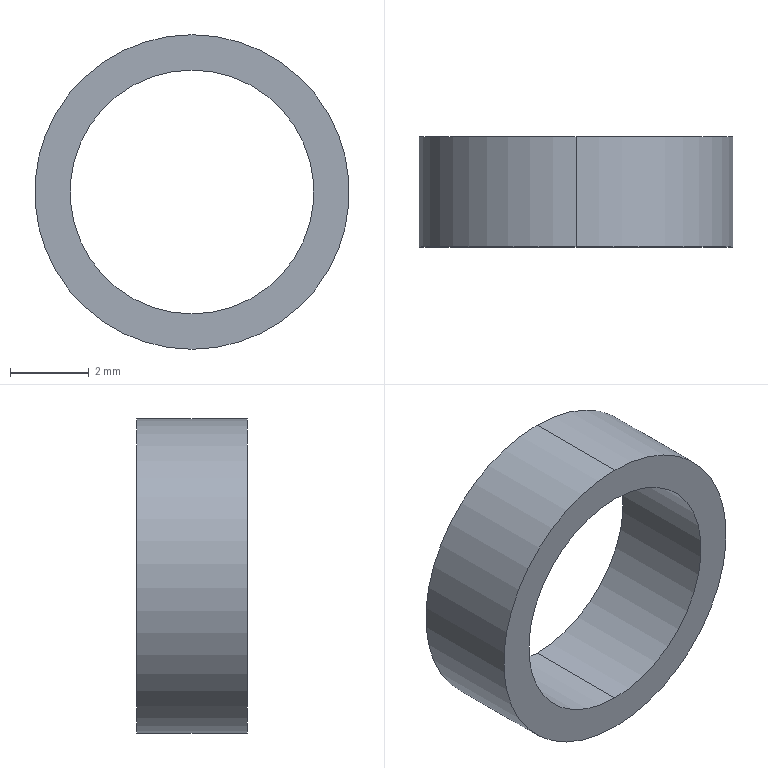Part | SolidWorks | features Extrusion 1 | 1 solid | 6 faces | box 8 x 2.8 x 8 mm | volume 56.209 mm3 | cylinder 4 | plane 2 | commonest cylinder face diameters 6.2 x2 8 x2
STEP:
#1=CARTESIAN_POINT('',(0.,2.8,-3.1));
#2=VERTEX_POINT('',#1);
#3=CARTESIAN_POINT('',(0.,2.8,3.1));
#4=VERTEX_POINT('',#3);
#5=CARTESIAN_POINT('',(0.,2.8,0.));
#6=DIRECTION('',(0.,1.,0.));
#7=DIRECTION('',(0.,0.,1.));
#8=AXIS2_PLACEMENT_3D('',#5,#6,#7);
#9=CIRCLE('',#8,3.1);
#10=EDGE_CURVE('',#2,#4,#9,.T.);
#11=ORIENTED_EDGE('',*,*,#10,.T.);
#12=CARTESIAN_POINT('',(0.,0.,3.1));
#13=VERTEX_POINT('',#12);
#14=CARTESIAN_POINT('',(0.,2.8,3.1));
#15=DIRECTION('',(0.,-1.,0.));
#16=VECTOR('',#15,1000.);
#17=LINE('',#14,#16);
#18=EDGE_CURVE('',#4,#13,#17,.T.);
#19=ORIENTED_EDGE('',*,*,#18,.T.);
#20=CARTESIAN_POINT('',(0.,0.,-3.1));
#21=VERTEX_POINT('',#20);
#22=CARTESIAN_POINT('',(0.,0.,0.));
#23=DIRECTION('',(0.,1.,0.));
#24=DIRECTION('',(0.,0.,1.));
#25=AXIS2_PLACEMENT_3D('',#22,#23,#24);
#26=CIRCLE('',#25,3.1);
#27=EDGE_CURVE('',#21,#13,#26,.T.);
#28=ORIENTED_EDGE('',*,*,#27,.F.);
#29=CARTESIAN_POINT('',(0.,2.8,-3.1));
#30=DIRECTION('',(0.,-1.,0.));
#31=VECTOR('',#30,1000.);
#32=LINE('',#29,#31);
#33=EDGE_CURVE('',#2,#21,#32,.T.);
#34=ORIENTED_EDGE('',*,*,#33,.F.);
#35=EDGE_LOOP('',(#11,#19,#28,#34));
#36=FACE_OUTER_BOUND('',#35,.T.);
#37=CARTESIAN_POINT('',(0.,2.8,0.));
#38=DIRECTION('',(0.,-1.,0.));
#39=DIRECTION('',(0.,0.,-1.));
#40=AXIS2_PLACEMENT_3D('',#37,#38,#39);
#41=CYLINDRICAL_SURFACE('',#40,3.1);
#42=ADVANCED_FACE('',(#36),#41,.F.);
#43=CARTESIAN_POINT('',(0.,2.8,4.));
#44=VERTEX_POINT('',#43);
#45=CARTESIAN_POINT('',(0.,2.8,-4.));
#46=VERTEX_POINT('',#45);
#47=CARTESIAN_POINT('',(0.,2.8,0.));
#48=DIRECTION('',(0.,1.,0.));
#49=DIRECTION('',(0.,0.,1.));
#50=AXIS2_PLACEMENT_3D('',#47,#48,#49);
#51=CIRCLE('',#50,4.);
#52=EDGE_CURVE('',#44,#46,#51,.T.);
#53=ORIENTED_EDGE('',*,*,#52,.F.);
#54=CARTESIAN_POINT('',(0.,0.,4.));
#55=VERTEX_POINT('',#54);
#56=CARTESIAN_POINT('',(0.,2.8,4.));
#57=DIRECTION('',(0.,-1.,0.));
#58=VECTOR('',#57,1000.);
#59=LINE('',#56,#58);
#60=EDGE_CURVE('',#44,#55,#59,.T.);
#61=ORIENTED_EDGE('',*,*,#60,.T.);
#62=CARTESIAN_POINT('',(0.,0.,-4.));
#63=VERTEX_POINT('',#62);
#64=CARTESIAN_POINT('',(0.,0.,0.));
#65=DIRECTION('',(0.,1.,0.));
#66=DIRECTION('',(0.,0.,1.));
#67=AXIS2_PLACEMENT_3D('',#64,#65,#66);
#68=CIRCLE('',#67,4.);
#69=EDGE_CURVE('',#55,#63,#68,.T.);
#70=ORIENTED_EDGE('',*,*,#69,.T.);
#71=CARTESIAN_POINT('',(0.,2.8,-4.));
#72=DIRECTION('',(0.,-1.,0.));
#73=VECTOR('',#72,1000.);
#74=LINE('',#71,#73);
#75=EDGE_CURVE('',#46,#63,#74,.T.);
#76=ORIENTED_EDGE('',*,*,#75,.F.);
#77=EDGE_LOOP('',(#53,#61,#70,#76));
#78=FACE_OUTER_BOUND('',#77,.T.);
#79=CARTESIAN_POINT('',(0.,2.8,0.));
#80=DIRECTION('',(0.,-1.,0.));
#81=DIRECTION('',(0.,0.,-1.));
#82=AXIS2_PLACEMENT_3D('',#79,#80,#81);
#83=CYLINDRICAL_SURFACE('',#82,4.);
#84=ADVANCED_FACE('',(#78),#83,.T.);
#85=CARTESIAN_POINT('',(0.,2.8,0.));
#86=DIRECTION('',(0.,1.,0.));
#87=DIRECTION('',(0.,0.,1.));
#88=AXIS2_PLACEMENT_3D('',#85,#86,#87);
#89=CIRCLE('',#88,4.);
#90=EDGE_CURVE('',#46,#44,#89,.T.);
#91=ORIENTED_EDGE('',*,*,#90,.T.);
#92=ORIENTED_EDGE('',*,*,#52,.T.);
#93=EDGE_LOOP('',(#91,#92));
#94=FACE_OUTER_BOUND('',#93,.T.);
#95=ORIENTED_EDGE('',*,*,#10,.F.);
#96=CARTESIAN_POINT('',(0.,2.8,0.));
#97=DIRECTION('',(0.,1.,0.));
#98=DIRECTION('',(0.,0.,1.));
#99=AXIS2_PLACEMENT_3D('',#96,#97,#98);
#100=CIRCLE('',#99,3.1);
#101=EDGE_CURVE('',#4,#2,#100,.T.);
#102=ORIENTED_EDGE('',*,*,#101,.F.);
#103=EDGE_LOOP('',(#95,#102));
#104=FACE_BOUND('',#103,.T.);
#105=CARTESIAN_POINT('',(0.,2.8,0.));
#106=DIRECTION('',(0.,1.,0.));
#107=DIRECTION('',(0.,0.,1.));
#108=AXIS2_PLACEMENT_3D('',#105,#106,#107);
#109=PLANE('',#108);
#110=ADVANCED_FACE('',(#94,#104),#109,.T.);
#111=CARTESIAN_POINT('',(0.,0.,0.));
#112=DIRECTION('',(0.,1.,0.));
#113=DIRECTION('',(0.,0.,1.));
#114=AXIS2_PLACEMENT_3D('',#111,#112,#113);
#115=CIRCLE('',#114,4.);
#116=EDGE_CURVE('',#63,#55,#115,.T.);
#117=ORIENTED_EDGE('',*,*,#116,.F.);
#118=ORIENTED_EDGE('',*,*,#69,.F.);
#119=EDGE_LOOP('',(#117,#118));
#120=FACE_OUTER_BOUND('',#119,.T.);
#121=ORIENTED_EDGE('',*,*,#27,.T.);
#122=CARTESIAN_POINT('',(0.,0.,0.));
#123=DIRECTION('',(0.,1.,0.));
#124=DIRECTION('',(0.,0.,1.));
#125=AXIS2_PLACEMENT_3D('',#122,#123,#124);
#126=CIRCLE('',#125,3.1);
#127=EDGE_CURVE('',#13,#21,#126,.T.);
#128=ORIENTED_EDGE('',*,*,#127,.T.);
#129=EDGE_LOOP('',(#121,#128));
#130=FACE_BOUND('',#129,.T.);
#131=CARTESIAN_POINT('',(0.,0.,0.));
#132=DIRECTION('',(0.,1.,0.));
#133=DIRECTION('',(0.,0.,1.));
#134=AXIS2_PLACEMENT_3D('',#131,#132,#133);
#135=PLANE('',#134);
#136=ADVANCED_FACE('',(#120,#130),#135,.F.);
#137=ORIENTED_EDGE('',*,*,#60,.F.);
#138=ORIENTED_EDGE('',*,*,#90,.F.);
#139=ORIENTED_EDGE('',*,*,#75,.T.);
#140=ORIENTED_EDGE('',*,*,#116,.T.);
#141=EDGE_LOOP('',(#137,#138,#139,#140));
#142=FACE_OUTER_BOUND('',#141,.T.);
#143=CARTESIAN_POINT('',(0.,2.8,0.));
#144=DIRECTION('',(0.,-1.,0.));
#145=DIRECTION('',(0.,0.,-1.));
#146=AXIS2_PLACEMENT_3D('',#143,#144,#145);
#147=CYLINDRICAL_SURFACE('',#146,4.);
#148=ADVANCED_FACE('',(#142),#147,.T.);
#149=ORIENTED_EDGE('',*,*,#18,.F.);
#150=ORIENTED_EDGE('',*,*,#101,.T.);
#151=ORIENTED_EDGE('',*,*,#33,.T.);
#152=ORIENTED_EDGE('',*,*,#127,.F.);
#153=EDGE_LOOP('',(#149,#150,#151,#152));
#154=FACE_OUTER_BOUND('',#153,.T.);
#155=CARTESIAN_POINT('',(0.,2.8,0.));
#156=DIRECTION('',(0.,-1.,0.));
#157=DIRECTION('',(0.,0.,-1.));
#158=AXIS2_PLACEMENT_3D('',#155,#156,#157);
#159=CYLINDRICAL_SURFACE('',#158,3.1);
#160=ADVANCED_FACE('',(#154),#159,.F.);
#161=CLOSED_SHELL('',(#42,#84,#110,#136,#148,#160));
#162=MANIFOLD_SOLID_BREP('',#161);
#163=CARTESIAN_POINT('',(0.,0.,0.));
#164=DIRECTION('',(0.,0.,1.));
#165=DIRECTION('',(1.,0.,0.));
#166=AXIS2_PLACEMENT_3D('',#163,#164,#165);
#167=(LENGTH_UNIT()NAMED_UNIT(*)SI_UNIT(.MILLI.,.METRE.));
#168=UNCERTAINTY_MEASURE_WITH_UNIT(LENGTH_MEASURE(0.00001),#167,'','');
#169=(NAMED_UNIT(*)PLANE_ANGLE_UNIT()SI_UNIT($,.RADIAN.));
#170=(NAMED_UNIT(*)SI_UNIT($,.STERADIAN.)SOLID_ANGLE_UNIT());
#171=(GEOMETRIC_REPRESENTATION_CONTEXT(3)GLOBAL_UNCERTAINTY_ASSIGNED_CONTEXT((#168))GLOBAL_UNIT_ASSIGNED_CONTEXT((#167,#169,#170))REPRESENTATION_CONTEXT('',''));
#172=ADVANCED_BREP_SHAPE_REPRESENTATION('',(#162,#166),#171);